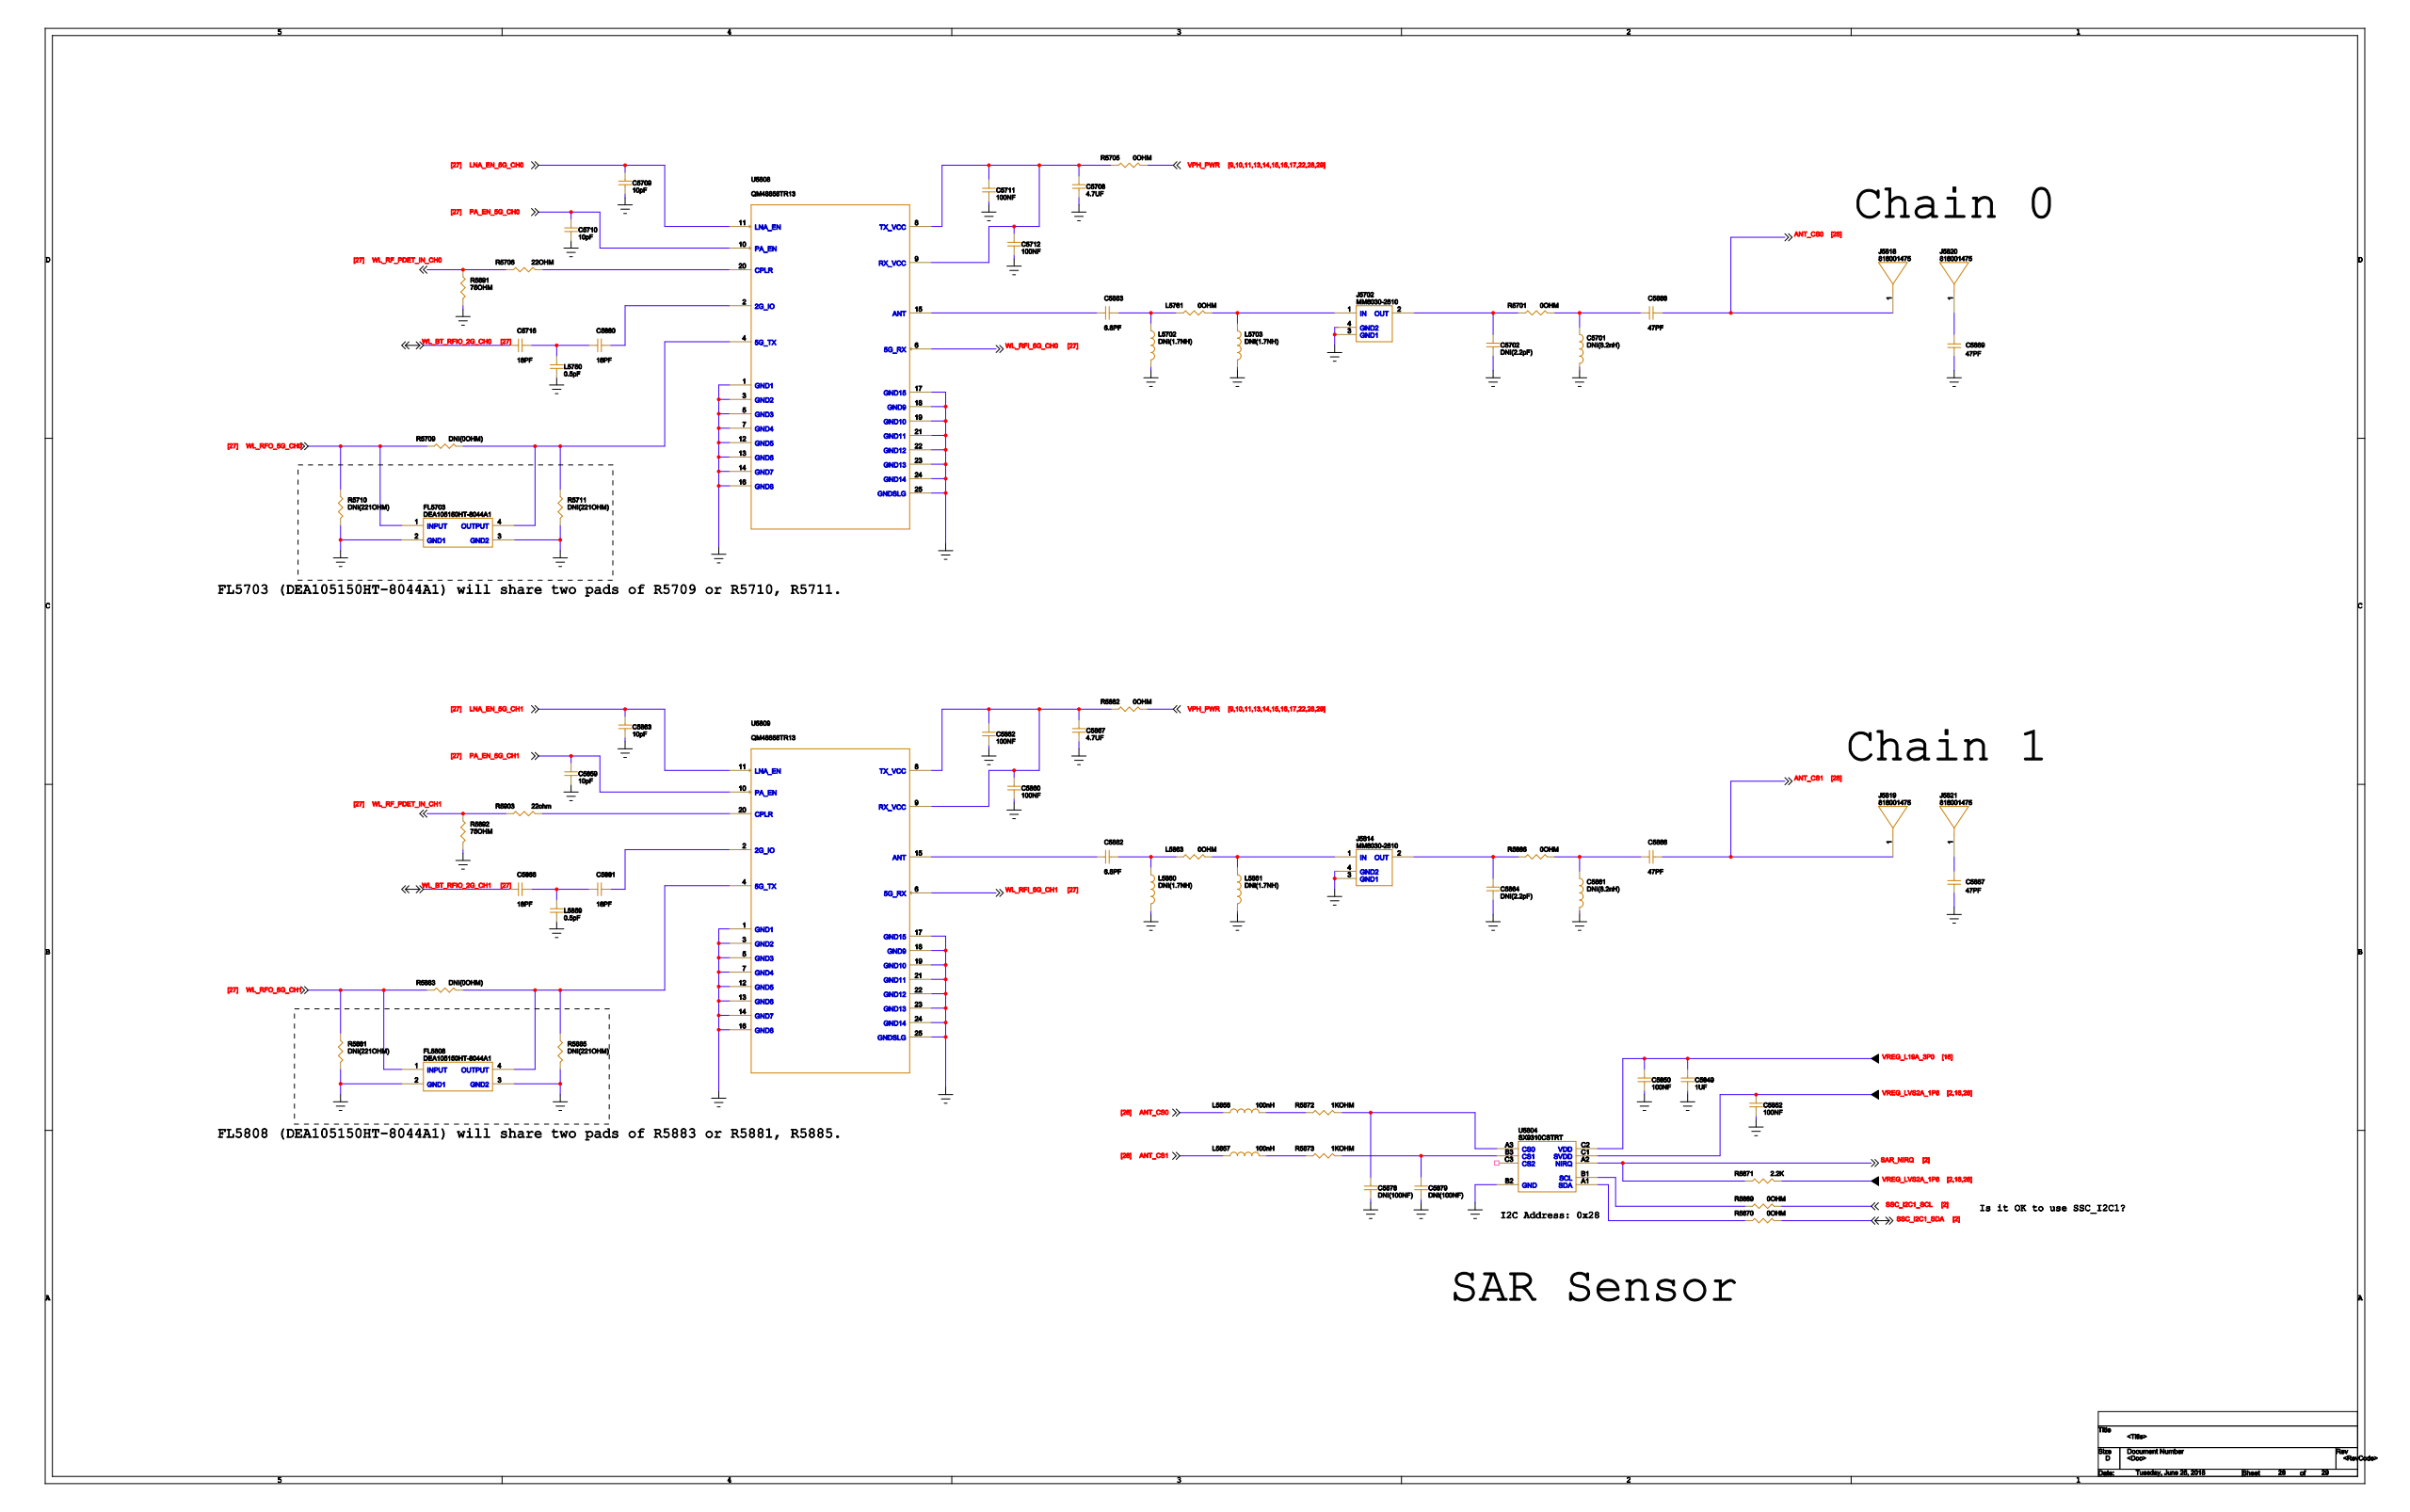Circuit board | Cadence Allegro | 802 parts | 566 nets | one sheet of the schematic
Parts on this sheet (reference | value | footprint):
C5701 | DNI(8.2nH) | L0201
C5702 | DNI(2.2pF) | C0201
C5708 | 4.7uF | 0402-BIG
C5709 | 10pF | C0201
C5710 | 10pF | C0201
C5711 | 100NF | C0201
C5712 | 100NF | C0201
C5716 | 18PF | C0201
C5849 | 1uF | C0201
C5850 | 100NF | C0201
C5852 | 100NF | C0201
C5859 | 10pF | C0201
C5860 | 100NF | C0201
C5861 | DNI(8.2nH) | L0201
C5862 | 100NF | C0201
C5863 | 10pF | C0201
C5864 | DNI(2.2pF) | C0201
C5866 | 18PF | C0201
C5867 | 4.7uF | 0402-BIG
C5878 | DNI(100NF) | C0201
C5879 | DNI(100NF) | C0201
C5880 | 18PF | C0201
C5881 | 18PF | C0201
C5882 | 6.8PF | C0201
C5883 | 6.8PF | C0201
C5886 | 47PF | C0201
C5887 | 47PF | C0201
C5888 | 47PF | C0201
C5889 | 47PF | C0201
FL5703 | DEA105150HT-8044A1 | DEA105150HT-8044A1
FL5808 | DEA105150HT-8044A1 | DEA105150HT-8044A1
J5702 | MM8030-2610 | RF_MM8030-2610
J5814 | MM8030-2610 | RF_MM8030-2610
J5818 | 818001475 | PIN_ANT_818001475
J5819 | 818001475 | PIN_ANT_818001475
J5820 | 818001475 | PIN_ANT_818001475
J5821 | 818001475 | PIN_ANT_818001475
L5702 | DNI(1.7NH) | L0201
L5703 | DNI(1.7NH) | L0201
L5750 | 0.5pF | C0201
L5761 | 0OHM | R0201
L5856 | 100nH | L0402
L5857 | 100nH | L0402
L5859 | 0.5pF | C0201
L5860 | DNI(1.7NH) | L0201
L5861 | DNI(1.7NH) | L0201
L5863 | 0OHM | R0201
R5701 | 0OHM | R0201
R5705 | 0OHM | R0402
R5706 | 22OHM | R0402
R5709 | DNI(0OHM) | R0201
R5710 | DNI(221OHM) | R0201
R5711 | DNI(221OHM) | R0201
R5869 | 0OHM | R0201
R5870 | 0OHM | R0201
R5871 | 2.2K | R0201
R5872 | 1KOHM | R0201
R5873 | 1KOHM | R0201
R5881 | DNI(221OHM) | R0201
R5882 | 0OHM | R0402
R5883 | DNI(0OHM) | R0201
R5885 | DNI(221OHM) | R0201
R5886 | 0OHM | R0201
R5891 | 75OHM | R0402
R5892 | 75OHM | R0402
R5903 | 22OHM | R0402
U5804 | SX9310CSTRT | WLCSP9_1P33X1P36X0P72_0P4
U5808 | QM48858TR13 | QFN24_3X3X0P798_0P4
U5809 | QM48858TR13 | QFN24_3X3X0P798_0P4
Nets of these parts (net: part-pin ...):
GND: C5701-2 C5702-2 C5708-2 C5709-2 C5710-2 C5711-2 C5712-2 C5849-2 C5850-2 C5852-2 C5859-2 C5860-2 C5861-2 C5862-2 C5863-2 C5864-2 C5867-2 C5878-2 C5879-2 C5887-1 C5889-1 FL5703-2 FL5703-3 FL5808-2 FL5808-3 J5702-3 J5702-4 J5814-3 J5814-4 L5702-2 L5703-2 L5750-2 L5859-2 L5860-2 L5861-2 R5710-2 R5711-2 R5881-2 R5885-2 R5891-2 R5892-2 U5804-B2 U5808-1 U5808-3 U5808-5 U5808-7 U5808-12 U5808-13 U5808-14 U5808-16 U5808-17 U5808-18 U5808-19 U5808-21 U5808-22 U5808-23 U5808-24 U5808-25 U5809-1 U5809-3 U5809-5 U5809-7 U5809-12 U5809-13 U5809-14 U5809-16 U5809-17 U5809-18 U5809-19 U5809-21 U5809-22 U5809-23 U5809-24 U5809-25
WL_RFO_5G_CH0: FL5703-1 R5709-1 R5710-1
N1108037: FL5703-4 R5709-2 R5711-1 U5808-4
WL_RFO_5G_CH1: FL5808-1 R5881-1 R5883-1
N1107019: FL5808-4 R5883-2 R5885-1 U5809-4
VPH_PWR: R5705-2 R5882-2
N1107567: C5708-1 C5711-1 C5712-1 R5705-1 U5808-8 U5808-9
VREG_L19A_3P0: C5849-1 C5850-1 U5804-C2
VREG_LVS2A_1P8: C5852-1 R5871-2 U5804-C1
N1109239: C5860-1 C5862-1 C5867-1 R5882-1 U5809-8 U5809-9
N1106871: C5887-2 J5821-1
N1108247: C5701-1 C5888-1 R5701-2
ANT_CS0: C5888-2 J5818-1 L5856-1
N1106779: C5861-1 C5886-1 R5886-2
ANT_CS1: C5886-2 J5819-1 L5857-1
N1108399: C5889-2 J5820-1
WL_RF_PDET_IN_CH0: R5706-1 R5891-1
WL_RF_PDET_IN_CH1: R5892-1 R5903-1
N1107733: C5878-1 R5872-2 U5804-A3
N1107843: C5879-1 R5873-2 U5804-B3
N1108235: C5702-1 J5702-2 R5701-1
N1106767: C5864-1 J5814-2 R5886-1
LNA_EN_5G_CH0: C5709-1 U5808-11
PA_EN_5G_CH0: C5710-1 U5808-10
PA_EN_5G_CH1: C5859-1 U5809-10
LNA_EN_5G_CH1: C5863-1 U5809-11
WL_BT_RFIO_2G_CH0: C5716-1
N1107531: C5716-2 C5880-1 L5750-1
WL_BT_RFIO_2G_CH1: C5866-1
N1109203: C5866-2 C5881-1 L5859-1
N1107471: C5880-2 U5808-2
N1109143: C5881-2 U5809-2
N1106661: C5882-1 U5809-15
N1106665: C5882-2 L5860-1 L5863-1
N1108017: C5883-1 U5808-15
N1108021: C5883-2 L5702-1 L5761-1
N1108029: J5702-1 L5703-1 L5761-2
N1106673: J5814-1 L5861-1 L5863-2
N1107803: R5869-1 U5804-B1
SSC_I2C1_SCL: R5869-2
N1107815: R5870-1 U5804-A1
SSC_I2C1_SDA: R5870-2
N1107737: L5856-2 R5872-1
N1107863: L5857-2 R5873-1
SAR_NIRQ: R5871-1 U5804-A2
N1107055: R5903-2 U5809-20
N1108729: R5706-2 U5808-20
WL_RFI_5G_CH0: U5808-6
WL_RFI_5G_CH1: U5809-6